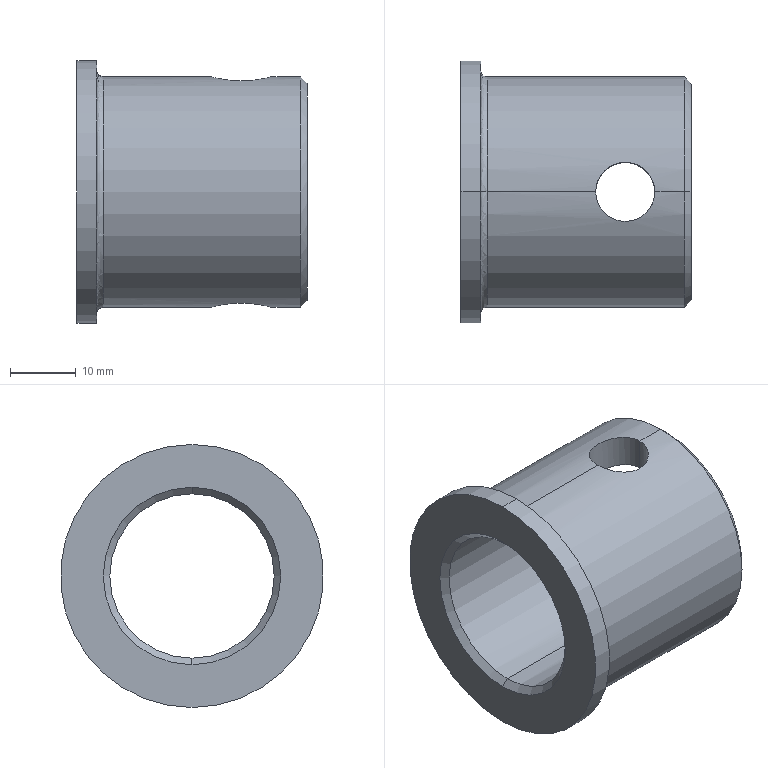Part | SolidWorks | features BaseBody 1 | 1 solid | 21 faces | box 35 x 40 x 40 mm | volume 16618 mm3 | cylinder 10 | cone 6 | plane 3 | spline 2 | commonest cylinder face diameters 9 x4 25 x2 35 x2 40 x2